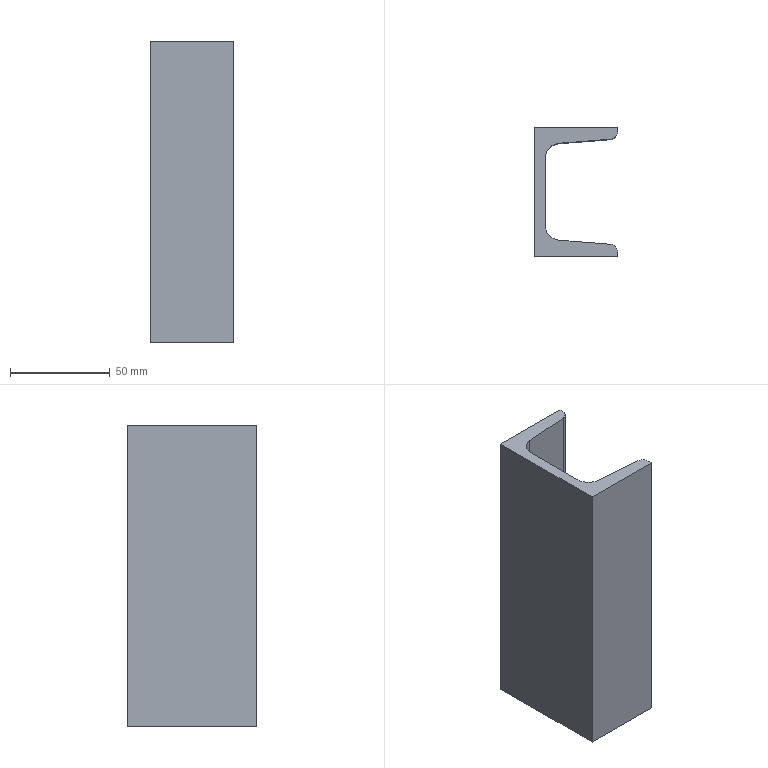Part | STEP file | DIN 1026-1 U 65 1785416005761 | 1 solid | 14 faces | box 42 x 65 x 150.668 mm | volume 136091 mm3 | plane 10 | cylinder 4 | commonest cylinder face diameters 8 x2 15 x2
STEP:
#1=CARTESIAN_POINT('',(5.5,-16.836,150.668));
#2=VERTEX_POINT('',#1);
#3=CARTESIAN_POINT('',(12.402,-24.312,150.668));
#4=VERTEX_POINT('',#3);
#5=CARTESIAN_POINT('',(13.,-16.836,150.668));
#6=DIRECTION('',(0.,0.,1.));
#7=DIRECTION('',(-1.,0.,0.));
#8=AXIS2_PLACEMENT_3D('',#5,#6,#7);
#9=CIRCLE('',#8,7.5);
#10=EDGE_CURVE('',#2,#4,#9,.T.);
#11=ORIENTED_EDGE('',*,*,#10,.T.);
#12=CARTESIAN_POINT('',(12.402,-24.312,0.));
#13=VERTEX_POINT('',#12);
#14=CARTESIAN_POINT('',(12.402,-24.312,0.));
#15=DIRECTION('',(0.,0.,1.));
#16=VECTOR('',#15,10.);
#17=LINE('',#14,#16);
#18=EDGE_CURVE('',#13,#4,#17,.T.);
#19=ORIENTED_EDGE('',*,*,#18,.F.);
#20=CARTESIAN_POINT('',(5.5,-16.836,0.));
#21=VERTEX_POINT('',#20);
#22=CARTESIAN_POINT('',(13.,-16.836,0.));
#23=DIRECTION('',(0.,0.,1.));
#24=DIRECTION('',(-1.,0.,0.));
#25=AXIS2_PLACEMENT_3D('',#22,#23,#24);
#26=CIRCLE('',#25,7.5);
#27=EDGE_CURVE('',#21,#13,#26,.T.);
#28=ORIENTED_EDGE('',*,*,#27,.F.);
#29=CARTESIAN_POINT('',(5.5,-16.836,0.));
#30=DIRECTION('',(0.,0.,1.));
#31=VECTOR('',#30,10.);
#32=LINE('',#29,#31);
#33=EDGE_CURVE('',#21,#2,#32,.T.);
#34=ORIENTED_EDGE('',*,*,#33,.T.);
#35=EDGE_LOOP('',(#11,#19,#28,#34));
#36=FACE_OUTER_BOUND('',#35,.T.);
#37=CARTESIAN_POINT('',(13.,-16.836,0.));
#38=DIRECTION('',(0.,0.,1.));
#39=DIRECTION('',(-1.,0.,0.));
#40=AXIS2_PLACEMENT_3D('',#37,#38,#39);
#41=CYLINDRICAL_SURFACE('',#40,7.5);
#42=ADVANCED_FACE('',(#36),#41,.F.);
#43=CARTESIAN_POINT('',(38.319,-26.386,150.668));
#44=VERTEX_POINT('',#43);
#45=CARTESIAN_POINT('',(15.707,-24.577,150.668));
#46=DIRECTION('',(0.9968,-0.07975,0.));
#47=VECTOR('',#46,10.);
#48=LINE('',#45,#47);
#49=EDGE_CURVE('',#4,#44,#48,.T.);
#50=ORIENTED_EDGE('',*,*,#49,.T.);
#51=CARTESIAN_POINT('',(38.319,-26.386,0.));
#52=VERTEX_POINT('',#51);
#53=CARTESIAN_POINT('',(38.319,-26.386,0.));
#54=DIRECTION('',(0.,0.,1.));
#55=VECTOR('',#54,10.);
#56=LINE('',#53,#55);
#57=EDGE_CURVE('',#52,#44,#56,.T.);
#58=ORIENTED_EDGE('',*,*,#57,.F.);
#59=CARTESIAN_POINT('',(15.707,-24.577,0.));
#60=DIRECTION('',(0.9968,-0.07975,0.));
#61=VECTOR('',#60,10.);
#62=LINE('',#59,#61);
#63=EDGE_CURVE('',#13,#52,#62,.T.);
#64=ORIENTED_EDGE('',*,*,#63,.F.);
#65=ORIENTED_EDGE('',*,*,#18,.T.);
#66=EDGE_LOOP('',(#50,#58,#64,#65));
#67=FACE_OUTER_BOUND('',#66,.T.);
#68=CARTESIAN_POINT('',(12.402,-24.312,0.));
#69=DIRECTION('',(0.07975,0.9968,0.));
#70=DIRECTION('',(0.,0.,1.));
#71=AXIS2_PLACEMENT_3D('',#68,#69,#70);
#72=PLANE('',#71);
#73=ADVANCED_FACE('',(#67),#72,.T.);
#74=CARTESIAN_POINT('',(42.,-30.373,150.668));
#75=VERTEX_POINT('',#74);
#76=CARTESIAN_POINT('',(38.,-30.373,150.668));
#77=DIRECTION('',(0.,0.,-1.));
#78=DIRECTION('',(-1.,0.,0.));
#79=AXIS2_PLACEMENT_3D('',#76,#77,#78);
#80=CIRCLE('',#79,4.);
#81=EDGE_CURVE('',#44,#75,#80,.T.);
#82=ORIENTED_EDGE('',*,*,#81,.T.);
#83=CARTESIAN_POINT('',(42.,-30.373,0.));
#84=VERTEX_POINT('',#83);
#85=CARTESIAN_POINT('',(42.,-30.373,0.));
#86=DIRECTION('',(0.,0.,1.));
#87=VECTOR('',#86,10.);
#88=LINE('',#85,#87);
#89=EDGE_CURVE('',#84,#75,#88,.T.);
#90=ORIENTED_EDGE('',*,*,#89,.F.);
#91=CARTESIAN_POINT('',(38.,-30.373,0.));
#92=DIRECTION('',(0.,0.,-1.));
#93=DIRECTION('',(-1.,0.,0.));
#94=AXIS2_PLACEMENT_3D('',#91,#92,#93);
#95=CIRCLE('',#94,4.);
#96=EDGE_CURVE('',#52,#84,#95,.T.);
#97=ORIENTED_EDGE('',*,*,#96,.F.);
#98=ORIENTED_EDGE('',*,*,#57,.T.);
#99=EDGE_LOOP('',(#82,#90,#97,#98));
#100=FACE_OUTER_BOUND('',#99,.T.);
#101=CARTESIAN_POINT('',(38.,-30.373,0.));
#102=DIRECTION('',(0.,0.,1.));
#103=DIRECTION('',(-1.,0.,0.));
#104=AXIS2_PLACEMENT_3D('',#101,#102,#103);
#105=CYLINDRICAL_SURFACE('',#104,4.);
#106=ADVANCED_FACE('',(#100),#105,.T.);
#107=CARTESIAN_POINT('',(42.,-32.5,150.668));
#108=VERTEX_POINT('',#107);
#109=CARTESIAN_POINT('',(42.,-15.186,150.668));
#110=DIRECTION('',(0.,-1.,0.));
#111=VECTOR('',#110,10.);
#112=LINE('',#109,#111);
#113=EDGE_CURVE('',#75,#108,#112,.T.);
#114=ORIENTED_EDGE('',*,*,#113,.T.);
#115=CARTESIAN_POINT('',(42.,-32.5,0.));
#116=VERTEX_POINT('',#115);
#117=CARTESIAN_POINT('',(42.,-32.5,0.));
#118=DIRECTION('',(0.,0.,1.));
#119=VECTOR('',#118,10.);
#120=LINE('',#117,#119);
#121=EDGE_CURVE('',#116,#108,#120,.T.);
#122=ORIENTED_EDGE('',*,*,#121,.F.);
#123=CARTESIAN_POINT('',(42.,-15.186,0.));
#124=DIRECTION('',(0.,-1.,0.));
#125=VECTOR('',#124,10.);
#126=LINE('',#123,#125);
#127=EDGE_CURVE('',#84,#116,#126,.T.);
#128=ORIENTED_EDGE('',*,*,#127,.F.);
#129=ORIENTED_EDGE('',*,*,#89,.T.);
#130=EDGE_LOOP('',(#114,#122,#128,#129));
#131=FACE_OUTER_BOUND('',#130,.T.);
#132=CARTESIAN_POINT('',(42.,-30.373,0.));
#133=DIRECTION('',(1.,0.,0.));
#134=DIRECTION('',(0.,0.,-1.));
#135=AXIS2_PLACEMENT_3D('',#132,#133,#134);
#136=PLANE('',#135);
#137=ADVANCED_FACE('',(#131),#136,.T.);
#138=CARTESIAN_POINT('',(0.,-32.5,150.668));
#139=VERTEX_POINT('',#138);
#140=CARTESIAN_POINT('',(31.5,-32.5,150.668));
#141=DIRECTION('',(-1.,0.,0.));
#142=VECTOR('',#141,10.);
#143=LINE('',#140,#142);
#144=EDGE_CURVE('',#108,#139,#143,.T.);
#145=ORIENTED_EDGE('',*,*,#144,.T.);
#146=CARTESIAN_POINT('',(0.,-32.5,0.));
#147=VERTEX_POINT('',#146);
#148=CARTESIAN_POINT('',(0.,-32.5,0.));
#149=DIRECTION('',(0.,0.,1.));
#150=VECTOR('',#149,10.);
#151=LINE('',#148,#150);
#152=EDGE_CURVE('',#147,#139,#151,.T.);
#153=ORIENTED_EDGE('',*,*,#152,.F.);
#154=CARTESIAN_POINT('',(31.5,-32.5,0.));
#155=DIRECTION('',(-1.,0.,0.));
#156=VECTOR('',#155,10.);
#157=LINE('',#154,#156);
#158=EDGE_CURVE('',#116,#147,#157,.T.);
#159=ORIENTED_EDGE('',*,*,#158,.F.);
#160=ORIENTED_EDGE('',*,*,#121,.T.);
#161=EDGE_LOOP('',(#145,#153,#159,#160));
#162=FACE_OUTER_BOUND('',#161,.T.);
#163=CARTESIAN_POINT('',(42.,-32.5,0.));
#164=DIRECTION('',(0.,-1.,0.));
#165=DIRECTION('',(0.,0.,-1.));
#166=AXIS2_PLACEMENT_3D('',#163,#164,#165);
#167=PLANE('',#166);
#168=ADVANCED_FACE('',(#162),#167,.T.);
#169=CARTESIAN_POINT('',(0.,32.5,150.668));
#170=VERTEX_POINT('',#169);
#171=CARTESIAN_POINT('',(0.,0.,150.668));
#172=DIRECTION('',(0.,1.,0.));
#173=VECTOR('',#172,10.);
#174=LINE('',#171,#173);
#175=EDGE_CURVE('',#139,#170,#174,.T.);
#176=ORIENTED_EDGE('',*,*,#175,.T.);
#177=CARTESIAN_POINT('',(0.,32.5,0.));
#178=VERTEX_POINT('',#177);
#179=CARTESIAN_POINT('',(0.,32.5,0.));
#180=DIRECTION('',(0.,0.,1.));
#181=VECTOR('',#180,10.);
#182=LINE('',#179,#181);
#183=EDGE_CURVE('',#178,#170,#182,.T.);
#184=ORIENTED_EDGE('',*,*,#183,.F.);
#185=CARTESIAN_POINT('',(0.,0.,0.));
#186=DIRECTION('',(0.,1.,0.));
#187=VECTOR('',#186,10.);
#188=LINE('',#185,#187);
#189=EDGE_CURVE('',#147,#178,#188,.T.);
#190=ORIENTED_EDGE('',*,*,#189,.F.);
#191=ORIENTED_EDGE('',*,*,#152,.T.);
#192=EDGE_LOOP('',(#176,#184,#190,#191));
#193=FACE_OUTER_BOUND('',#192,.T.);
#194=CARTESIAN_POINT('',(0.,0.,0.));
#195=DIRECTION('',(-1.,0.,0.));
#196=DIRECTION('',(0.,0.,1.));
#197=AXIS2_PLACEMENT_3D('',#194,#195,#196);
#198=PLANE('',#197);
#199=ADVANCED_FACE('',(#193),#198,.T.);
#200=CARTESIAN_POINT('',(42.,32.5,150.668));
#201=VERTEX_POINT('',#200);
#202=CARTESIAN_POINT('',(10.5,32.5,150.668));
#203=DIRECTION('',(1.,0.,0.));
#204=VECTOR('',#203,10.);
#205=LINE('',#202,#204);
#206=EDGE_CURVE('',#170,#201,#205,.T.);
#207=ORIENTED_EDGE('',*,*,#206,.T.);
#208=CARTESIAN_POINT('',(42.,32.5,0.));
#209=VERTEX_POINT('',#208);
#210=CARTESIAN_POINT('',(42.,32.5,0.));
#211=DIRECTION('',(0.,0.,1.));
#212=VECTOR('',#211,10.);
#213=LINE('',#210,#212);
#214=EDGE_CURVE('',#209,#201,#213,.T.);
#215=ORIENTED_EDGE('',*,*,#214,.F.);
#216=CARTESIAN_POINT('',(10.5,32.5,0.));
#217=DIRECTION('',(1.,0.,0.));
#218=VECTOR('',#217,10.);
#219=LINE('',#216,#218);
#220=EDGE_CURVE('',#178,#209,#219,.T.);
#221=ORIENTED_EDGE('',*,*,#220,.F.);
#222=ORIENTED_EDGE('',*,*,#183,.T.);
#223=EDGE_LOOP('',(#207,#215,#221,#222));
#224=FACE_OUTER_BOUND('',#223,.T.);
#225=CARTESIAN_POINT('',(0.,32.5,0.));
#226=DIRECTION('',(0.,1.,0.));
#227=DIRECTION('',(0.,0.,1.));
#228=AXIS2_PLACEMENT_3D('',#225,#226,#227);
#229=PLANE('',#228);
#230=ADVANCED_FACE('',(#224),#229,.T.);
#231=CARTESIAN_POINT('',(42.,30.373,150.668));
#232=VERTEX_POINT('',#231);
#233=CARTESIAN_POINT('',(42.,16.25,150.668));
#234=DIRECTION('',(0.,-1.,0.));
#235=VECTOR('',#234,10.);
#236=LINE('',#233,#235);
#237=EDGE_CURVE('',#201,#232,#236,.T.);
#238=ORIENTED_EDGE('',*,*,#237,.T.);
#239=CARTESIAN_POINT('',(42.,30.373,0.));
#240=VERTEX_POINT('',#239);
#241=CARTESIAN_POINT('',(42.,30.373,0.));
#242=DIRECTION('',(0.,0.,1.));
#243=VECTOR('',#242,10.);
#244=LINE('',#241,#243);
#245=EDGE_CURVE('',#240,#232,#244,.T.);
#246=ORIENTED_EDGE('',*,*,#245,.F.);
#247=CARTESIAN_POINT('',(42.,16.25,0.));
#248=DIRECTION('',(0.,-1.,0.));
#249=VECTOR('',#248,10.);
#250=LINE('',#247,#249);
#251=EDGE_CURVE('',#209,#240,#250,.T.);
#252=ORIENTED_EDGE('',*,*,#251,.F.);
#253=ORIENTED_EDGE('',*,*,#214,.T.);
#254=EDGE_LOOP('',(#238,#246,#252,#253));
#255=FACE_OUTER_BOUND('',#254,.T.);
#256=CARTESIAN_POINT('',(42.,32.5,0.));
#257=DIRECTION('',(1.,0.,0.));
#258=DIRECTION('',(0.,0.,-1.));
#259=AXIS2_PLACEMENT_3D('',#256,#257,#258);
#260=PLANE('',#259);
#261=ADVANCED_FACE('',(#255),#260,.T.);
#262=CARTESIAN_POINT('',(38.319,26.386,150.668));
#263=VERTEX_POINT('',#262);
#264=CARTESIAN_POINT('',(38.,30.373,150.668));
#265=DIRECTION('',(0.,0.,-1.));
#266=DIRECTION('',(-0.07975,0.9968,0.));
#267=AXIS2_PLACEMENT_3D('',#264,#265,#266);
#268=CIRCLE('',#267,4.);
#269=EDGE_CURVE('',#232,#263,#268,.T.);
#270=ORIENTED_EDGE('',*,*,#269,.T.);
#271=CARTESIAN_POINT('',(38.319,26.386,0.));
#272=VERTEX_POINT('',#271);
#273=CARTESIAN_POINT('',(38.319,26.386,0.));
#274=DIRECTION('',(0.,0.,1.));
#275=VECTOR('',#274,10.);
#276=LINE('',#273,#275);
#277=EDGE_CURVE('',#272,#263,#276,.T.);
#278=ORIENTED_EDGE('',*,*,#277,.F.);
#279=CARTESIAN_POINT('',(38.,30.373,0.));
#280=DIRECTION('',(0.,0.,-1.));
#281=DIRECTION('',(-0.07975,0.9968,0.));
#282=AXIS2_PLACEMENT_3D('',#279,#280,#281);
#283=CIRCLE('',#282,4.);
#284=EDGE_CURVE('',#240,#272,#283,.T.);
#285=ORIENTED_EDGE('',*,*,#284,.F.);
#286=ORIENTED_EDGE('',*,*,#245,.T.);
#287=EDGE_LOOP('',(#270,#278,#285,#286));
#288=FACE_OUTER_BOUND('',#287,.T.);
#289=CARTESIAN_POINT('',(38.,30.373,0.));
#290=DIRECTION('',(0.,0.,1.));
#291=DIRECTION('',(-0.07975,0.9968,0.));
#292=AXIS2_PLACEMENT_3D('',#289,#290,#291);
#293=CYLINDRICAL_SURFACE('',#292,4.);
#294=ADVANCED_FACE('',(#288),#293,.T.);
#295=CARTESIAN_POINT('',(12.402,24.312,150.668));
#296=VERTEX_POINT('',#295);
#297=CARTESIAN_POINT('',(28.666,25.613,150.668));
#298=DIRECTION('',(-0.9968,-0.07975,0.));
#299=VECTOR('',#298,10.);
#300=LINE('',#297,#299);
#301=EDGE_CURVE('',#263,#296,#300,.T.);
#302=ORIENTED_EDGE('',*,*,#301,.T.);
#303=CARTESIAN_POINT('',(12.402,24.312,0.));
#304=VERTEX_POINT('',#303);
#305=CARTESIAN_POINT('',(12.402,24.312,0.));
#306=DIRECTION('',(0.,0.,1.));
#307=VECTOR('',#306,10.);
#308=LINE('',#305,#307);
#309=EDGE_CURVE('',#304,#296,#308,.T.);
#310=ORIENTED_EDGE('',*,*,#309,.F.);
#311=CARTESIAN_POINT('',(28.666,25.613,0.));
#312=DIRECTION('',(-0.9968,-0.07975,0.));
#313=VECTOR('',#312,10.);
#314=LINE('',#311,#313);
#315=EDGE_CURVE('',#272,#304,#314,.T.);
#316=ORIENTED_EDGE('',*,*,#315,.F.);
#317=ORIENTED_EDGE('',*,*,#277,.T.);
#318=EDGE_LOOP('',(#302,#310,#316,#317));
#319=FACE_OUTER_BOUND('',#318,.T.);
#320=CARTESIAN_POINT('',(38.319,26.386,0.));
#321=DIRECTION('',(0.07975,-0.9968,0.));
#322=DIRECTION('',(0.,0.,-1.));
#323=AXIS2_PLACEMENT_3D('',#320,#321,#322);
#324=PLANE('',#323);
#325=ADVANCED_FACE('',(#319),#324,.T.);
#326=CARTESIAN_POINT('',(5.5,16.836,150.668));
#327=VERTEX_POINT('',#326);
#328=CARTESIAN_POINT('',(13.,16.836,150.668));
#329=DIRECTION('',(0.,0.,1.));
#330=DIRECTION('',(-0.07975,0.9968,0.));
#331=AXIS2_PLACEMENT_3D('',#328,#329,#330);
#332=CIRCLE('',#331,7.5);
#333=EDGE_CURVE('',#296,#327,#332,.T.);
#334=ORIENTED_EDGE('',*,*,#333,.T.);
#335=CARTESIAN_POINT('',(5.5,16.836,0.));
#336=VERTEX_POINT('',#335);
#337=CARTESIAN_POINT('',(5.5,16.836,0.));
#338=DIRECTION('',(0.,0.,1.));
#339=VECTOR('',#338,10.);
#340=LINE('',#337,#339);
#341=EDGE_CURVE('',#336,#327,#340,.T.);
#342=ORIENTED_EDGE('',*,*,#341,.F.);
#343=CARTESIAN_POINT('',(13.,16.836,0.));
#344=DIRECTION('',(0.,0.,1.));
#345=DIRECTION('',(-0.07975,0.9968,0.));
#346=AXIS2_PLACEMENT_3D('',#343,#344,#345);
#347=CIRCLE('',#346,7.5);
#348=EDGE_CURVE('',#304,#336,#347,.T.);
#349=ORIENTED_EDGE('',*,*,#348,.F.);
#350=ORIENTED_EDGE('',*,*,#309,.T.);
#351=EDGE_LOOP('',(#334,#342,#349,#350));
#352=FACE_OUTER_BOUND('',#351,.T.);
#353=CARTESIAN_POINT('',(13.,16.836,0.));
#354=DIRECTION('',(0.,0.,1.));
#355=DIRECTION('',(-0.07975,0.9968,0.));
#356=AXIS2_PLACEMENT_3D('',#353,#354,#355);
#357=CYLINDRICAL_SURFACE('',#356,7.5);
#358=ADVANCED_FACE('',(#352),#357,.F.);
#359=CARTESIAN_POINT('',(5.5,0.,150.668));
#360=DIRECTION('',(0.,-1.,0.));
#361=VECTOR('',#360,10.);
#362=LINE('',#359,#361);
#363=EDGE_CURVE('',#327,#2,#362,.T.);
#364=ORIENTED_EDGE('',*,*,#363,.T.);
#365=ORIENTED_EDGE('',*,*,#33,.F.);
#366=CARTESIAN_POINT('',(5.5,0.,0.));
#367=DIRECTION('',(0.,-1.,0.));
#368=VECTOR('',#367,10.);
#369=LINE('',#366,#368);
#370=EDGE_CURVE('',#336,#21,#369,.T.);
#371=ORIENTED_EDGE('',*,*,#370,.F.);
#372=ORIENTED_EDGE('',*,*,#341,.T.);
#373=EDGE_LOOP('',(#364,#365,#371,#372));
#374=FACE_OUTER_BOUND('',#373,.T.);
#375=CARTESIAN_POINT('',(5.5,0.,0.));
#376=DIRECTION('',(1.,0.,0.));
#377=DIRECTION('',(0.,0.,-1.));
#378=AXIS2_PLACEMENT_3D('',#375,#376,#377);
#379=PLANE('',#378);
#380=ADVANCED_FACE('',(#374),#379,.T.);
#381=ORIENTED_EDGE('',*,*,#220,.T.);
#382=ORIENTED_EDGE('',*,*,#251,.T.);
#383=ORIENTED_EDGE('',*,*,#284,.T.);
#384=ORIENTED_EDGE('',*,*,#315,.T.);
#385=ORIENTED_EDGE('',*,*,#348,.T.);
#386=ORIENTED_EDGE('',*,*,#370,.T.);
#387=ORIENTED_EDGE('',*,*,#27,.T.);
#388=ORIENTED_EDGE('',*,*,#63,.T.);
#389=ORIENTED_EDGE('',*,*,#96,.T.);
#390=ORIENTED_EDGE('',*,*,#127,.T.);
#391=ORIENTED_EDGE('',*,*,#158,.T.);
#392=ORIENTED_EDGE('',*,*,#189,.T.);
#393=EDGE_LOOP('',(#381,#382,#383,#384,#385,#386,#387,#388,#389,#390,#391,#392));
#394=FACE_OUTER_BOUND('',#393,.T.);
#395=CARTESIAN_POINT('',(21.,0.,0.));
#396=DIRECTION('',(0.,0.,1.));
#397=DIRECTION('',(1.,0.,0.));
#398=AXIS2_PLACEMENT_3D('',#395,#396,#397);
#399=PLANE('',#398);
#400=ADVANCED_FACE('',(#394),#399,.F.);
#401=ORIENTED_EDGE('',*,*,#206,.F.);
#402=ORIENTED_EDGE('',*,*,#175,.F.);
#403=ORIENTED_EDGE('',*,*,#144,.F.);
#404=ORIENTED_EDGE('',*,*,#113,.F.);
#405=ORIENTED_EDGE('',*,*,#81,.F.);
#406=ORIENTED_EDGE('',*,*,#49,.F.);
#407=ORIENTED_EDGE('',*,*,#10,.F.);
#408=ORIENTED_EDGE('',*,*,#363,.F.);
#409=ORIENTED_EDGE('',*,*,#333,.F.);
#410=ORIENTED_EDGE('',*,*,#301,.F.);
#411=ORIENTED_EDGE('',*,*,#269,.F.);
#412=ORIENTED_EDGE('',*,*,#237,.F.);
#413=EDGE_LOOP('',(#401,#402,#403,#404,#405,#406,#407,#408,#409,#410,#411,#412));
#414=FACE_OUTER_BOUND('',#413,.T.);
#415=CARTESIAN_POINT('',(21.,0.,150.668));
#416=DIRECTION('',(0.,0.,1.));
#417=DIRECTION('',(1.,0.,0.));
#418=AXIS2_PLACEMENT_3D('',#415,#416,#417);
#419=PLANE('',#418);
#420=ADVANCED_FACE('',(#414),#419,.T.);
#421=CLOSED_SHELL('',(#42,#73,#106,#137,#168,#199,#230,#261,#294,#325,#358,#380,#400,#420));
#422=MANIFOLD_SOLID_BREP('',#421);
#423=(LENGTH_UNIT()NAMED_UNIT(*)SI_UNIT(.MILLI.,.METRE.));
#424=UNCERTAINTY_MEASURE_WITH_UNIT(LENGTH_MEASURE(0.01),#423,'','');
#425=(NAMED_UNIT(*)PLANE_ANGLE_UNIT()SI_UNIT($,.RADIAN.));
#426=(NAMED_UNIT(*)SI_UNIT($,.STERADIAN.)SOLID_ANGLE_UNIT());
#427=(GEOMETRIC_REPRESENTATION_CONTEXT(3)GLOBAL_UNCERTAINTY_ASSIGNED_CONTEXT((#424))GLOBAL_UNIT_ASSIGNED_CONTEXT((#423,#425,#426))REPRESENTATION_CONTEXT('',''));
#428=ADVANCED_BREP_SHAPE_REPRESENTATION('',(#422),#427);